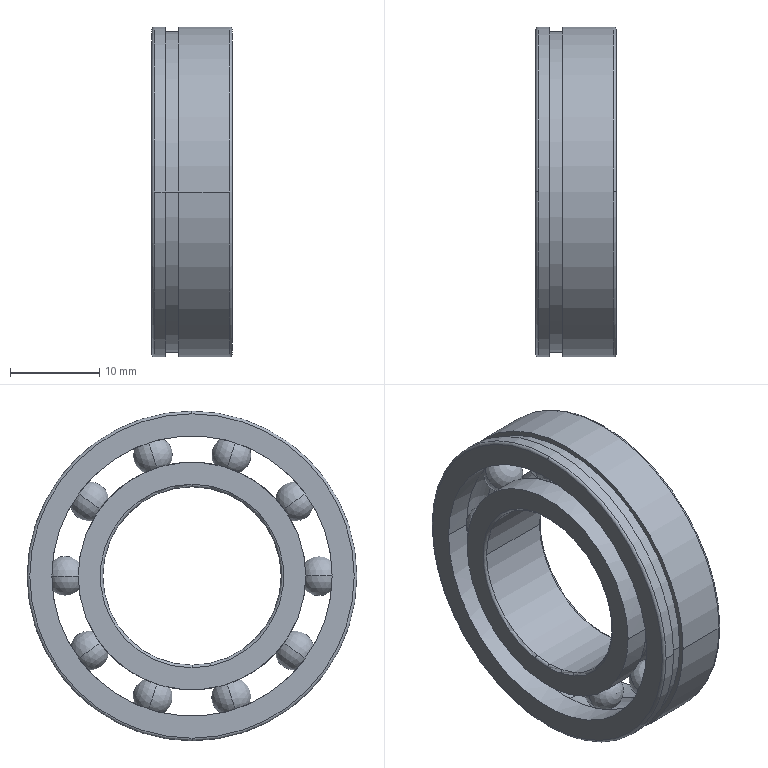Part | SolidWorks | features BaseBody 12 | 12 solids | 56 faces | box 9 x 37 x 37 mm | volume 4521 mm3 | sphere 20 | cylinder 16 | torus 14 | plane 6 | commonest cylinder face diameters 25.542 x4 31.458 x4 37 x4 20 x2 35.92 x2
STEP:
#1=CARTESIAN_POINT('',(4.5,12.04,0.));
#2=VERTEX_POINT('',#1);
#3=CARTESIAN_POINT('',(4.5,16.46,0.));
#4=VERTEX_POINT('',#3);
#5=CARTESIAN_POINT('',(4.5,14.25,0.));
#6=DIRECTION('',(0.,0.,1.));
#7=DIRECTION('',(1.,0.,0.));
#8=AXIS2_PLACEMENT_3D('',#5,#6,#7);
#9=CIRCLE('',#8,2.21);
#10=EDGE_CURVE('',#2,#4,#9,.T.);
#11=ORIENTED_EDGE('',*,*,#10,.F.);
#12=CARTESIAN_POINT('',(4.5,14.25,0.));
#13=DIRECTION('',(0.,0.,-1.));
#14=DIRECTION('',(-1.,0.,0.));
#15=AXIS2_PLACEMENT_3D('',#12,#13,#14);
#16=CIRCLE('',#15,2.21);
#17=EDGE_CURVE('',#2,#4,#16,.T.);
#18=ORIENTED_EDGE('',*,*,#17,.T.);
#19=EDGE_LOOP('',(#11,#18));
#20=FACE_OUTER_BOUND('',#19,.T.);
#21=CARTESIAN_POINT('',(4.5,14.25,0.));
#22=DIRECTION('',(0.,0.,-1.));
#23=DIRECTION('',(1.,0.,0.));
#24=AXIS2_PLACEMENT_3D('',#21,#22,#23);
#25=SPHERICAL_SURFACE('',#24,2.21);
#26=ADVANCED_FACE('',(#20),#25,.T.);
#27=ORIENTED_EDGE('',*,*,#17,.F.);
#28=ORIENTED_EDGE('',*,*,#10,.T.);
#29=EDGE_LOOP('',(#27,#28));
#30=FACE_OUTER_BOUND('',#29,.T.);
#31=CARTESIAN_POINT('',(4.5,14.25,0.));
#32=DIRECTION('',(0.,0.,-1.));
#33=DIRECTION('',(1.,0.,0.));
#34=AXIS2_PLACEMENT_3D('',#31,#32,#33);
#35=SPHERICAL_SURFACE('',#34,2.21);
#36=ADVANCED_FACE('',(#30),#35,.T.);
#37=CLOSED_SHELL('',(#26,#36));
#38=MANIFOLD_SOLID_BREP('',#37);
#39=CARTESIAN_POINT('',(3.,-17.96,0.));
#40=VERTEX_POINT('',#39);
#41=CARTESIAN_POINT('',(3.,17.96,0.));
#42=VERTEX_POINT('',#41);
#43=CARTESIAN_POINT('',(3.,0.,0.));
#44=DIRECTION('',(1.,0.,0.));
#45=DIRECTION('',(0.,1.,0.));
#46=AXIS2_PLACEMENT_3D('',#43,#44,#45);
#47=CIRCLE('',#46,17.96);
#48=EDGE_CURVE('',#40,#42,#47,.T.);
#49=ORIENTED_EDGE('',*,*,#48,.F.);
#50=CARTESIAN_POINT('',(1.5,-17.96,0.));
#51=VERTEX_POINT('',#50);
#52=CARTESIAN_POINT('',(2.25,-17.96,0.));
#53=DIRECTION('',(-1.,0.,0.));
#54=VECTOR('',#53,1000.);
#55=LINE('',#52,#54);
#56=EDGE_CURVE('',#40,#51,#55,.T.);
#57=ORIENTED_EDGE('',*,*,#56,.T.);
#58=CARTESIAN_POINT('',(1.5,17.96,0.));
#59=VERTEX_POINT('',#58);
#60=CARTESIAN_POINT('',(1.5,0.,0.));
#61=DIRECTION('',(1.,0.,0.));
#62=DIRECTION('',(0.,1.,0.));
#63=AXIS2_PLACEMENT_3D('',#60,#61,#62);
#64=CIRCLE('',#63,17.96);
#65=EDGE_CURVE('',#51,#59,#64,.T.);
#66=ORIENTED_EDGE('',*,*,#65,.T.);
#67=CARTESIAN_POINT('',(2.25,17.96,0.));
#68=DIRECTION('',(-1.,0.,0.));
#69=VECTOR('',#68,1000.);
#70=LINE('',#67,#69);
#71=EDGE_CURVE('',#42,#59,#70,.T.);
#72=ORIENTED_EDGE('',*,*,#71,.F.);
#73=EDGE_LOOP('',(#49,#57,#66,#72));
#74=FACE_OUTER_BOUND('',#73,.T.);
#75=CARTESIAN_POINT('',(2.25,0.,0.));
#76=DIRECTION('',(-1.,0.,0.));
#77=DIRECTION('',(0.,1.,0.));
#78=AXIS2_PLACEMENT_3D('',#75,#76,#77);
#79=CYLINDRICAL_SURFACE('',#78,17.96);
#80=ADVANCED_FACE('',(#74),#79,.T.);
#81=CARTESIAN_POINT('',(8.7,-18.5,0.));
#82=VERTEX_POINT('',#81);
#83=CARTESIAN_POINT('',(8.7,0.,-18.5));
#84=VERTEX_POINT('',#83);
#85=CARTESIAN_POINT('',(8.7,0.,0.));
#86=DIRECTION('',(1.,0.,0.));
#87=DIRECTION('',(0.,-1.,0.));
#88=AXIS2_PLACEMENT_3D('',#85,#86,#87);
#89=CIRCLE('',#88,18.5);
#90=EDGE_CURVE('',#82,#84,#89,.T.);
#91=ORIENTED_EDGE('',*,*,#90,.F.);
#92=CARTESIAN_POINT('',(3.,-18.5,0.));
#93=VERTEX_POINT('',#92);
#94=CARTESIAN_POINT('',(6.,-18.5,0.));
#95=DIRECTION('',(-1.,0.,0.));
#96=VECTOR('',#95,1000.);
#97=LINE('',#94,#96);
#98=EDGE_CURVE('',#82,#93,#97,.T.);
#99=ORIENTED_EDGE('',*,*,#98,.T.);
#100=CARTESIAN_POINT('',(3.,18.5,0.));
#101=VERTEX_POINT('',#100);
#102=CARTESIAN_POINT('',(3.,0.,0.));
#103=DIRECTION('',(1.,0.,0.));
#104=DIRECTION('',(0.,1.,0.));
#105=AXIS2_PLACEMENT_3D('',#102,#103,#104);
#106=CIRCLE('',#105,18.5);
#107=EDGE_CURVE('',#93,#101,#106,.T.);
#108=ORIENTED_EDGE('',*,*,#107,.T.);
#109=CARTESIAN_POINT('',(8.7,18.5,0.));
#110=VERTEX_POINT('',#109);
#111=CARTESIAN_POINT('',(6.,18.5,0.));
#112=DIRECTION('',(-1.,0.,0.));
#113=VECTOR('',#112,1000.);
#114=LINE('',#111,#113);
#115=EDGE_CURVE('',#110,#101,#114,.T.);
#116=ORIENTED_EDGE('',*,*,#115,.F.);
#117=CARTESIAN_POINT('',(8.7,0.,0.));
#118=DIRECTION('',(1.,0.,0.));
#119=DIRECTION('',(0.,-1.,0.));
#120=AXIS2_PLACEMENT_3D('',#117,#118,#119);
#121=CIRCLE('',#120,18.5);
#122=EDGE_CURVE('',#84,#110,#121,.T.);
#123=ORIENTED_EDGE('',*,*,#122,.F.);
#124=EDGE_LOOP('',(#91,#99,#108,#116,#123));
#125=FACE_OUTER_BOUND('',#124,.T.);
#126=CARTESIAN_POINT('',(6.,0.,0.));
#127=DIRECTION('',(-1.,0.,0.));
#128=DIRECTION('',(0.,1.,0.));
#129=AXIS2_PLACEMENT_3D('',#126,#127,#128);
#130=CYLINDRICAL_SURFACE('',#129,18.5);
#131=ADVANCED_FACE('',(#125),#130,.T.);
#132=CARTESIAN_POINT('',(1.5,-18.5,0.));
#133=VERTEX_POINT('',#132);
#134=CARTESIAN_POINT('',(1.5,18.5,0.));
#135=VERTEX_POINT('',#134);
#136=CARTESIAN_POINT('',(1.5,0.,0.));
#137=DIRECTION('',(1.,0.,0.));
#138=DIRECTION('',(0.,1.,0.));
#139=AXIS2_PLACEMENT_3D('',#136,#137,#138);
#140=CIRCLE('',#139,18.5);
#141=EDGE_CURVE('',#133,#135,#140,.T.);
#142=ORIENTED_EDGE('',*,*,#141,.F.);
#143=CARTESIAN_POINT('',(0.3,-18.5,0.));
#144=VERTEX_POINT('',#143);
#145=CARTESIAN_POINT('',(0.75,-18.5,0.));
#146=DIRECTION('',(-1.,0.,0.));
#147=VECTOR('',#146,1000.);
#148=LINE('',#145,#147);
#149=EDGE_CURVE('',#133,#144,#148,.T.);
#150=ORIENTED_EDGE('',*,*,#149,.T.);
#151=CARTESIAN_POINT('',(0.3,0.,-18.5));
#152=VERTEX_POINT('',#151);
#153=CARTESIAN_POINT('',(0.3,0.,0.));
#154=DIRECTION('',(-1.,0.,0.));
#155=DIRECTION('',(0.,-1.,0.));
#156=AXIS2_PLACEMENT_3D('',#153,#154,#155);
#157=CIRCLE('',#156,18.5);
#158=EDGE_CURVE('',#152,#144,#157,.T.);
#159=ORIENTED_EDGE('',*,*,#158,.F.);
#160=CARTESIAN_POINT('',(0.3,18.5,0.));
#161=VERTEX_POINT('',#160);
#162=CARTESIAN_POINT('',(0.3,0.,0.));
#163=DIRECTION('',(-1.,0.,0.));
#164=DIRECTION('',(0.,-1.,0.));
#165=AXIS2_PLACEMENT_3D('',#162,#163,#164);
#166=CIRCLE('',#165,18.5);
#167=EDGE_CURVE('',#161,#152,#166,.T.);
#168=ORIENTED_EDGE('',*,*,#167,.F.);
#169=CARTESIAN_POINT('',(0.75,18.5,0.));
#170=DIRECTION('',(-1.,0.,0.));
#171=VECTOR('',#170,1000.);
#172=LINE('',#169,#171);
#173=EDGE_CURVE('',#135,#161,#172,.T.);
#174=ORIENTED_EDGE('',*,*,#173,.F.);
#175=EDGE_LOOP('',(#142,#150,#159,#168,#174));
#176=FACE_OUTER_BOUND('',#175,.T.);
#177=CARTESIAN_POINT('',(0.75,0.,0.));
#178=DIRECTION('',(-1.,0.,0.));
#179=DIRECTION('',(0.,1.,0.));
#180=AXIS2_PLACEMENT_3D('',#177,#178,#179);
#181=CYLINDRICAL_SURFACE('',#180,18.5);
#182=ADVANCED_FACE('',(#176),#181,.T.);
#183=ORIENTED_EDGE('',*,*,#122,.T.);
#184=CARTESIAN_POINT('',(8.7,0.,18.5));
#185=VERTEX_POINT('',#184);
#186=CARTESIAN_POINT('',(8.7,0.,0.));
#187=DIRECTION('',(1.,0.,0.));
#188=DIRECTION('',(0.,-1.,0.));
#189=AXIS2_PLACEMENT_3D('',#186,#187,#188);
#190=CIRCLE('',#189,18.5);
#191=EDGE_CURVE('',#110,#185,#190,.T.);
#192=ORIENTED_EDGE('',*,*,#191,.T.);
#193=CARTESIAN_POINT('',(9.,0.,18.2));
#194=VERTEX_POINT('',#193);
#195=CARTESIAN_POINT('',(8.7,0.,18.2));
#196=DIRECTION('',(0.,1.,0.));
#197=DIRECTION('',(0.,0.,1.));
#198=AXIS2_PLACEMENT_3D('',#195,#196,#197);
#199=CIRCLE('',#198,0.3);
#200=EDGE_CURVE('',#185,#194,#199,.T.);
#201=ORIENTED_EDGE('',*,*,#200,.T.);
#202=CARTESIAN_POINT('',(9.,0.,-18.2));
#203=VERTEX_POINT('',#202);
#204=CARTESIAN_POINT('',(9.,0.,0.));
#205=DIRECTION('',(-1.,0.,0.));
#206=DIRECTION('',(0.,-1.,0.));
#207=AXIS2_PLACEMENT_3D('',#204,#205,#206);
#208=CIRCLE('',#207,18.2);
#209=EDGE_CURVE('',#194,#203,#208,.T.);
#210=ORIENTED_EDGE('',*,*,#209,.T.);
#211=CARTESIAN_POINT('',(8.7,0.,-18.2));
#212=DIRECTION('',(0.,-1.,0.));
#213=DIRECTION('',(0.,0.,-1.));
#214=AXIS2_PLACEMENT_3D('',#211,#212,#213);
#215=CIRCLE('',#214,0.3);
#216=EDGE_CURVE('',#84,#203,#215,.T.);
#217=ORIENTED_EDGE('',*,*,#216,.F.);
#218=EDGE_LOOP('',(#183,#192,#201,#210,#217));
#219=FACE_OUTER_BOUND('',#218,.T.);
#220=CARTESIAN_POINT('',(8.7,0.,0.));
#221=DIRECTION('',(1.,0.,0.));
#222=DIRECTION('',(0.,0.,-1.));
#223=AXIS2_PLACEMENT_3D('',#220,#221,#222);
#224=TOROIDAL_SURFACE('',#223,18.2,0.3);
#225=ADVANCED_FACE('',(#219),#224,.T.);
#226=CARTESIAN_POINT('',(0.,0.,-18.2));
#227=VERTEX_POINT('',#226);
#228=CARTESIAN_POINT('',(0.,0.,18.2));
#229=VERTEX_POINT('',#228);
#230=CARTESIAN_POINT('',(0.,0.,0.));
#231=DIRECTION('',(1.,0.,0.));
#232=DIRECTION('',(0.,-1.,0.));
#233=AXIS2_PLACEMENT_3D('',#230,#231,#232);
#234=CIRCLE('',#233,18.2);
#235=EDGE_CURVE('',#227,#229,#234,.T.);
#236=ORIENTED_EDGE('',*,*,#235,.T.);
#237=CARTESIAN_POINT('',(0.3,0.,18.5));
#238=VERTEX_POINT('',#237);
#239=CARTESIAN_POINT('',(0.3,0.,18.2));
#240=DIRECTION('',(0.,1.,0.));
#241=DIRECTION('',(0.,0.,1.));
#242=AXIS2_PLACEMENT_3D('',#239,#240,#241);
#243=CIRCLE('',#242,0.3);
#244=EDGE_CURVE('',#229,#238,#243,.T.);
#245=ORIENTED_EDGE('',*,*,#244,.T.);
#246=CARTESIAN_POINT('',(0.3,0.,0.));
#247=DIRECTION('',(-1.,0.,0.));
#248=DIRECTION('',(0.,-1.,0.));
#249=AXIS2_PLACEMENT_3D('',#246,#247,#248);
#250=CIRCLE('',#249,18.5);
#251=EDGE_CURVE('',#238,#161,#250,.T.);
#252=ORIENTED_EDGE('',*,*,#251,.T.);
#253=ORIENTED_EDGE('',*,*,#167,.T.);
#254=CARTESIAN_POINT('',(0.3,0.,-18.2));
#255=DIRECTION('',(0.,-1.,0.));
#256=DIRECTION('',(0.,0.,-1.));
#257=AXIS2_PLACEMENT_3D('',#254,#255,#256);
#258=CIRCLE('',#257,0.3);
#259=EDGE_CURVE('',#227,#152,#258,.T.);
#260=ORIENTED_EDGE('',*,*,#259,.F.);
#261=EDGE_LOOP('',(#236,#245,#252,#253,#260));
#262=FACE_OUTER_BOUND('',#261,.T.);
#263=CARTESIAN_POINT('',(0.3,0.,0.));
#264=DIRECTION('',(1.,0.,0.));
#265=DIRECTION('',(0.,0.,-1.));
#266=AXIS2_PLACEMENT_3D('',#263,#264,#265);
#267=TOROIDAL_SURFACE('',#266,18.2,0.3);
#268=ADVANCED_FACE('',(#262),#267,.T.);
#269=CARTESIAN_POINT('',(2.858,0.,15.729));
#270=VERTEX_POINT('',#269);
#271=CARTESIAN_POINT('',(2.858,-15.729,0.));
#272=VERTEX_POINT('',#271);
#273=CARTESIAN_POINT('',(2.858,0.,0.));
#274=DIRECTION('',(1.,0.,0.));
#275=DIRECTION('',(0.,1.,0.));
#276=AXIS2_PLACEMENT_3D('',#273,#274,#275);
#277=CIRCLE('',#276,15.729);
#278=EDGE_CURVE('',#270,#272,#277,.T.);
#279=ORIENTED_EDGE('',*,*,#278,.F.);
#280=CARTESIAN_POINT('',(6.142,0.,15.729));
#281=VERTEX_POINT('',#280);
#282=CARTESIAN_POINT('',(4.5,0.,14.25));
#283=DIRECTION('',(0.,1.,0.));
#284=DIRECTION('',(0.,0.,1.));
#285=AXIS2_PLACEMENT_3D('',#282,#283,#284);
#286=CIRCLE('',#285,2.21);
#287=EDGE_CURVE('',#270,#281,#286,.T.);
#288=ORIENTED_EDGE('',*,*,#287,.T.);
#289=CARTESIAN_POINT('',(6.142,-15.729,0.));
#290=VERTEX_POINT('',#289);
#291=CARTESIAN_POINT('',(6.142,0.,0.));
#292=DIRECTION('',(1.,0.,0.));
#293=DIRECTION('',(0.,1.,0.));
#294=AXIS2_PLACEMENT_3D('',#291,#292,#293);
#295=CIRCLE('',#294,15.729);
#296=EDGE_CURVE('',#281,#290,#295,.T.);
#297=ORIENTED_EDGE('',*,*,#296,.T.);
#298=CARTESIAN_POINT('',(6.142,0.,-15.729));
#299=VERTEX_POINT('',#298);
#300=CARTESIAN_POINT('',(6.142,0.,0.));
#301=DIRECTION('',(1.,0.,0.));
#302=DIRECTION('',(0.,1.,0.));
#303=AXIS2_PLACEMENT_3D('',#300,#301,#302);
#304=CIRCLE('',#303,15.729);
#305=EDGE_CURVE('',#290,#299,#304,.T.);
#306=ORIENTED_EDGE('',*,*,#305,.T.);
#307=CARTESIAN_POINT('',(2.858,0.,-15.729));
#308=VERTEX_POINT('',#307);
#309=CARTESIAN_POINT('',(4.5,0.,-14.25));
#310=DIRECTION('',(0.,-1.,0.));
#311=DIRECTION('',(0.,0.,-1.));
#312=AXIS2_PLACEMENT_3D('',#309,#310,#311);
#313=CIRCLE('',#312,2.21);
#314=EDGE_CURVE('',#308,#299,#313,.T.);
#315=ORIENTED_EDGE('',*,*,#314,.F.);
#316=CARTESIAN_POINT('',(2.858,0.,0.));
#317=DIRECTION('',(1.,0.,0.));
#318=DIRECTION('',(0.,1.,0.));
#319=AXIS2_PLACEMENT_3D('',#316,#317,#318);
#320=CIRCLE('',#319,15.729);
#321=EDGE_CURVE('',#272,#308,#320,.T.);
#322=ORIENTED_EDGE('',*,*,#321,.F.);
#323=EDGE_LOOP('',(#279,#288,#297,#306,#315,#322));
#324=FACE_OUTER_BOUND('',#323,.T.);
#325=CARTESIAN_POINT('',(4.5,0.,0.));
#326=DIRECTION('',(1.,0.,0.));
#327=DIRECTION('',(0.,0.,-1.));
#328=AXIS2_PLACEMENT_3D('',#325,#326,#327);
#329=TOROIDAL_SURFACE('',#328,14.25,2.21);
#330=ADVANCED_FACE('',(#324),#329,.F.);
#331=CARTESIAN_POINT('',(9.,15.729,0.));
#332=VERTEX_POINT('',#331);
#333=CARTESIAN_POINT('',(9.,-15.729,0.));
#334=VERTEX_POINT('',#333);
#335=CARTESIAN_POINT('',(9.,0.,0.));
#336=DIRECTION('',(1.,0.,0.));
#337=DIRECTION('',(0.,1.,0.));
#338=AXIS2_PLACEMENT_3D('',#335,#336,#337);
#339=CIRCLE('',#338,15.729);
#340=EDGE_CURVE('',#332,#334,#339,.T.);
#341=ORIENTED_EDGE('',*,*,#340,.T.);
#342=CARTESIAN_POINT('',(7.571,-15.729,0.));
#343=DIRECTION('',(-1.,0.,0.));
#344=VECTOR('',#343,1000.);
#345=LINE('',#342,#344);
#346=EDGE_CURVE('',#334,#290,#345,.T.);
#347=ORIENTED_EDGE('',*,*,#346,.T.);
#348=ORIENTED_EDGE('',*,*,#296,.F.);
#349=CARTESIAN_POINT('',(6.142,15.729,0.));
#350=VERTEX_POINT('',#349);
#351=CARTESIAN_POINT('',(6.142,0.,0.));
#352=DIRECTION('',(1.,0.,0.));
#353=DIRECTION('',(0.,1.,0.));
#354=AXIS2_PLACEMENT_3D('',#351,#352,#353);
#355=CIRCLE('',#354,15.729);
#356=EDGE_CURVE('',#350,#281,#355,.T.);
#357=ORIENTED_EDGE('',*,*,#356,.F.);
#358=CARTESIAN_POINT('',(7.571,15.729,0.));
#359=DIRECTION('',(-1.,0.,0.));
#360=VECTOR('',#359,1000.);
#361=LINE('',#358,#360);
#362=EDGE_CURVE('',#332,#350,#361,.T.);
#363=ORIENTED_EDGE('',*,*,#362,.F.);
#364=EDGE_LOOP('',(#341,#347,#348,#357,#363));
#365=FACE_OUTER_BOUND('',#364,.T.);
#366=CARTESIAN_POINT('',(7.571,0.,0.));
#367=DIRECTION('',(-1.,0.,0.));
#368=DIRECTION('',(0.,1.,0.));
#369=AXIS2_PLACEMENT_3D('',#366,#367,#368);
#370=CYLINDRICAL_SURFACE('',#369,15.729);
#371=ADVANCED_FACE('',(#365),#370,.F.);
#372=CARTESIAN_POINT('',(2.858,15.729,0.));
#373=VERTEX_POINT('',#372);
#374=CARTESIAN_POINT('',(2.858,0.,0.));
#375=DIRECTION('',(1.,0.,0.));
#376=DIRECTION('',(0.,1.,0.));
#377=AXIS2_PLACEMENT_3D('',#374,#375,#376);
#378=CIRCLE('',#377,15.729);
#379=EDGE_CURVE('',#373,#270,#378,.T.);
#380=ORIENTED_EDGE('',*,*,#379,.T.);
#381=ORIENTED_EDGE('',*,*,#278,.T.);
#382=CARTESIAN_POINT('',(0.,-15.729,0.));
#383=VERTEX_POINT('',#382);
#384=CARTESIAN_POINT('',(1.429,-15.729,0.));
#385=DIRECTION('',(-1.,0.,0.));
#386=VECTOR('',#385,1000.);
#387=LINE('',#384,#386);
#388=EDGE_CURVE('',#272,#383,#387,.T.);
#389=ORIENTED_EDGE('',*,*,#388,.T.);
#390=CARTESIAN_POINT('',(0.,15.729,0.));
#391=VERTEX_POINT('',#390);
#392=CARTESIAN_POINT('',(0.,0.,0.));
#393=DIRECTION('',(1.,0.,0.));
#394=DIRECTION('',(0.,1.,0.));
#395=AXIS2_PLACEMENT_3D('',#392,#393,#394);
#396=CIRCLE('',#395,15.729);
#397=EDGE_CURVE('',#391,#383,#396,.T.);
#398=ORIENTED_EDGE('',*,*,#397,.F.);
#399=CARTESIAN_POINT('',(1.429,15.729,0.));
#400=DIRECTION('',(-1.,0.,0.));
#401=VECTOR('',#400,1000.);
#402=LINE('',#399,#401);
#403=EDGE_CURVE('',#373,#391,#402,.T.);
#404=ORIENTED_EDGE('',*,*,#403,.F.);
#405=EDGE_LOOP('',(#380,#381,#389,#398,#404));
#406=FACE_OUTER_BOUND('',#405,.T.);
#407=CARTESIAN_POINT('',(1.429,0.,0.));
#408=DIRECTION('',(-1.,0.,0.));
#409=DIRECTION('',(0.,1.,0.));
#410=AXIS2_PLACEMENT_3D('',#407,#408,#409);
#411=CYLINDRICAL_SURFACE('',#410,15.729);
#412=ADVANCED_FACE('',(#406),#411,.F.);
#413=CARTESIAN_POINT('',(3.,0.,0.));
#414=DIRECTION('',(1.,0.,0.));
#415=DIRECTION('',(0.,1.,0.));
#416=AXIS2_PLACEMENT_3D('',#413,#414,#415);
#417=CIRCLE('',#416,17.96);
#418=EDGE_CURVE('',#42,#40,#417,.T.);
#419=ORIENTED_EDGE('',*,*,#418,.T.);
#420=ORIENTED_EDGE('',*,*,#48,.T.);
#421=EDGE_LOOP('',(#419,#420));
#422=FACE_BOUND('',#421,.T.);
#423=CARTESIAN_POINT('',(3.,0.,0.));
#424=DIRECTION('',(1.,0.,0.));
#425=DIRECTION('',(0.,1.,0.));
#426=AXIS2_PLACEMENT_3D('',#423,#424,#425);
#427=CIRCLE('',#426,18.5);
#428=EDGE_CURVE('',#101,#93,#427,.T.);
#429=ORIENTED_EDGE('',*,*,#428,.F.);
#430=ORIENTED_EDGE('',*,*,#107,.F.);
#431=EDGE_LOOP('',(#429,#430));
#432=FACE_OUTER_BOUND('',#431,.T.);
#433=CARTESIAN_POINT('',(3.,18.23,0.));
#434=DIRECTION('',(-1.,0.,0.));
#435=DIRECTION('',(0.,0.,1.));
#436=AXIS2_PLACEMENT_3D('',#433,#434,#435);
#437=PLANE('',#436);
#438=ADVANCED_FACE('',(#422,#432),#437,.T.);
#439=CARTESIAN_POINT('',(1.5,0.,0.));
#440=DIRECTION('',(1.,0.,0.));
#441=DIRECTION('',(0.,1.,0.));
#442=AXIS2_PLACEMENT_3D('',#439,#440,#441);
#443=CIRCLE('',#442,17.96);
#444=EDGE_CURVE('',#59,#51,#443,.T.);
#445=ORIENTED_EDGE('',*,*,#444,.F.);
#446=ORIENTED_EDGE('',*,*,#65,.F.);
#447=EDGE_LOOP('',(#445,#446));
#448=FACE_BOUND('',#447,.T.);
#449=CARTESIAN_POINT('',(1.5,0.,0.));
#450=DIRECTION('',(1.,0.,0.));
#451=DIRECTION('',(0.,1.,0.));
#452=AXIS2_PLACEMENT_3D('',#449,#450,#451);
#453=CIRCLE('',#452,18.5);
#454=EDGE_CURVE('',#135,#133,#453,.T.);
#455=ORIENTED_EDGE('',*,*,#454,.T.);
#456=ORIENTED_EDGE('',*,*,#141,.T.);
#457=EDGE_LOOP('',(#455,#456));
#458=FACE_OUTER_BOUND('',#457,.T.);
#459=CARTESIAN_POINT('',(1.5,18.23,0.));
#460=DIRECTION('',(1.,0.,0.));
#461=DIRECTION('',(0.,1.,0.));
#462=AXIS2_PLACEMENT_3D('',#459,#460,#461);
#463=PLANE('',#462);
#464=ADVANCED_FACE('',(#448,#458),#463,.T.);
#465=ORIENTED_EDGE('',*,*,#340,.F.);
#466=CARTESIAN_POINT('',(9.,0.,0.));
#467=DIRECTION('',(1.,0.,0.));
#468=DIRECTION('',(0.,1.,0.));
#469=AXIS2_PLACEMENT_3D('',#466,#467,#468);
#470=CIRCLE('',#469,15.729);
#471=EDGE_CURVE('',#334,#332,#470,.T.);
#472=ORIENTED_EDGE('',*,*,#471,.F.);
#473=EDGE_LOOP('',(#465,#472));
#474=FACE_BOUND('',#473,.T.);
#475=CARTESIAN_POINT('',(9.,0.,0.));
#476=DIRECTION('',(-1.,0.,0.));
#477=DIRECTION('',(0.,-1.,0.));
#478=AXIS2_PLACEMENT_3D('',#475,#476,#477);
#479=CIRCLE('',#478,18.2);
#480=EDGE_CURVE('',#203,#194,#479,.T.);
#481=ORIENTED_EDGE('',*,*,#480,.F.);
#482=ORIENTED_EDGE('',*,*,#209,.F.);
#483=EDGE_LOOP('',(#481,#482));
#484=FACE_OUTER_BOUND('',#483,.T.);
#485=CARTESIAN_POINT('',(9.,17.114,0.));
#486=DIRECTION('',(1.,0.,0.));
#487=DIRECTION('',(0.,1.,0.));
#488=AXIS2_PLACEMENT_3D('',#485,#486,#487);
#489=PLANE('',#488);
#490=ADVANCED_FACE('',(#474,#484),#489,.T.);
#491=ORIENTED_EDGE('',*,*,#397,.T.);
#492=CARTESIAN_POINT('',(0.,0.,0.));
#493=DIRECTION('',(1.,0.,0.));
#494=DIRECTION('',(0.,1.,0.));
#495=AXIS2_PLACEMENT_3D('',#492,#493,#494);
#496=CIRCLE('',#495,15.729);
#497=EDGE_CURVE('',#383,#391,#496,.T.);
#498=ORIENTED_EDGE('',*,*,#497,.T.);
#499=EDGE_LOOP('',(#491,#498));
#500=FACE_BOUND('',#499,.T.);
#501=ORIENTED_EDGE('',*,*,#235,.F.);
#502=CARTESIAN_POINT('',(0.,0.,0.));
#503=DIRECTION('',(1.,0.,0.));
#504=DIRECTION('',(0.,-1.,0.));
#505=AXIS2_PLACEMENT_3D('',#502,#503,#504);
#506=CIRCLE('',#505,18.2);
#507=EDGE_CURVE('',#229,#227,#506,.T.);
#508=ORIENTED_EDGE('',*,*,#507,.F.);
#509=EDGE_LOOP('',(#501,#508));
#510=FACE_OUTER_BOUND('',#509,.T.);
#511=CARTESIAN_POINT('',(0.,17.114,0.));
#512=DIRECTION('',(-1.,0.,0.));
#513=DIRECTION('',(0.,0.,1.));
#514=AXIS2_PLACEMENT_3D('',#511,#512,#513);
#515=PLANE('',#514);
#516=ADVANCED_FACE('',(#500,#510),#515,.T.);
#517=ORIENTED_EDGE('',*,*,#388,.F.);
#518=ORIENTED_EDGE('',*,*,#321,.T.);
#519=CARTESIAN_POINT('',(2.858,0.,0.));
#520=DIRECTION('',(1.,0.,0.));
#521=DIRECTION('',(0.,1.,0.));
#522=AXIS2_PLACEMENT_3D('',#519,#520,#521);
#523=CIRCLE('',#522,15.729);
#524=EDGE_CURVE('',#308,#373,#523,.T.);
#525=ORIENTED_EDGE('',*,*,#524,.T.);
#526=ORIENTED_EDGE('',*,*,#403,.T.);
#527=ORIENTED_EDGE('',*,*,#497,.F.);
#528=EDGE_LOOP('',(#517,#518,#525,#526,#527));
#529=FACE_OUTER_BOUND('',#528,.T.);
#530=CARTESIAN_POINT('',(1.429,0.,0.));
#531=DIRECTION('',(-1.,0.,0.));
#532=DIRECTION('',(0.,1.,0.));
#533=AXIS2_PLACEMENT_3D('',#530,#531,#532);
#534=CYLINDRICAL_SURFACE('',#533,15.729);
#535=ADVANCED_FACE('',(#529),#534,.F.);
#536=ORIENTED_EDGE('',*,*,#346,.F.);
#537=ORIENTED_EDGE('',*,*,#471,.T.);
#538=ORIENTED_EDGE('',*,*,#362,.T.);
#539=CARTESIAN_POINT('',(6.142,0.,0.));
#540=DIRECTION('',(1.,0.,0.));
#541=DIRECTION('',(0.,1.,0.));
#542=AXIS2_PLACEMENT_3D('',#539,#540,#541);
#543=CIRCLE('',#542,15.729);
#544=EDGE_CURVE('',#299,#350,#543,.T.);
#545=ORIENTED_EDGE('',*,*,#544,.F.);
#546=ORIENTED_EDGE('',*,*,#305,.F.);
#547=EDGE_LOOP('',(#536,#537,#538,#545,#546));
#548=FACE_OUTER_BOUND('',#547,.T.);
#549=CARTESIAN_POINT('',(7.571,0.,0.));
#550=DIRECTION('',(-1.,0.,0.));
#551=DIRECTION('',(0.,1.,0.));
#552=AXIS2_PLACEMENT_3D('',#549,#550,#551);
#553=CYLINDRICAL_SURFACE('',#552,15.729);
#554=ADVANCED_FACE('',(#548),#553,.F.);
#555=ORIENTED_EDGE('',*,*,#287,.F.);
#556=ORIENTED_EDGE('',*,*,#379,.F.);
#557=ORIENTED_EDGE('',*,*,#524,.F.);
#558=ORIENTED_EDGE('',*,*,#314,.T.);
#559=ORIENTED_EDGE('',*,*,#544,.T.);
#560=ORIENTED_EDGE('',*,*,#356,.T.);
#561=EDGE_LOOP('',(#555,#556,#557,#558,#559,#560));
#562=FACE_OUTER_BOUND('',#561,.T.);
#563=CARTESIAN_POINT('',(4.5,0.,0.));
#564=DIRECTION('',(1.,0.,0.));
#565=DIRECTION('',(0.,0.,-1.));
#566=AXIS2_PLACEMENT_3D('',#563,#564,#565);
#567=TOROIDAL_SURFACE('',#566,14.25,2.21);
#568=ADVANCED_FACE('',(#562),#567,.F.);
#569=ORIENTED_EDGE('',*,*,#244,.F.);
#570=ORIENTED_EDGE('',*,*,#507,.T.);
#571=ORIENTED_EDGE('',*,*,#259,.T.);
#572=ORIENTED_EDGE('',*,*,#158,.T.);
#573=CARTESIAN_POINT('',(0.3,0.,0.));
#574=DIRECTION('',(-1.,0.,0.));
#575=DIRECTION('',(0.,-1.,0.));
#576=AXIS2_PLACEMENT_3D('',#573,#574,#575);
#577=CIRCLE('',#576,18.5);
#578=EDGE_CURVE('',#144,#238,#577,.T.);
#579=ORIENTED_EDGE('',*,*,#578,.T.);
#580=EDGE_LOOP('',(#569,#570,#571,#572,#579));
#581=FACE_OUTER_BOUND('',#580,.T.);
#582=CARTESIAN_POINT('',(0.3,0.,0.));
#583=DIRECTION('',(1.,0.,0.));
#584=DIRECTION('',(0.,0.,-1.));
#585=AXIS2_PLACEMENT_3D('',#582,#583,#584);
#586=TOROIDAL_SURFACE('',#585,18.2,0.3);
#587=ADVANCED_FACE('',(#581),#586,.T.);
#588=ORIENTED_EDGE('',*,*,#200,.F.);
#589=CARTESIAN_POINT('',(8.7,0.,0.));
#590=DIRECTION('',(1.,0.,0.));
#591=DIRECTION('',(0.,-1.,0.));
#592=AXIS2_PLACEMENT_3D('',#589,#590,#591);
#593=CIRCLE('',#592,18.5);
#594=EDGE_CURVE('',#185,#82,#593,.T.);
#595=ORIENTED_EDGE('',*,*,#594,.T.);
#596=ORIENTED_EDGE('',*,*,#90,.T.);
#597=ORIENTED_EDGE('',*,*,#216,.T.);
#598=ORIENTED_EDGE('',*,*,#480,.T.);
#599=EDGE_LOOP('',(#588,#595,#596,#597,#598));
#600=FACE_OUTER_BOUND('',#599,.T.);
#601=CARTESIAN_POINT('',(8.7,0.,0.));
#602=DIRECTION('',(1.,0.,0.));
#603=DIRECTION('',(0.,0.,-1.));
#604=AXIS2_PLACEMENT_3D('',#601,#602,#603);
#605=TOROIDAL_SURFACE('',#604,18.2,0.3);
#606=ADVANCED_FACE('',(#600),#605,.T.);
#607=ORIENTED_EDGE('',*,*,#149,.F.);
#608=ORIENTED_EDGE('',*,*,#454,.F.);
#609=ORIENTED_EDGE('',*,*,#173,.T.);
#610=ORIENTED_EDGE('',*,*,#251,.F.);
#611=ORIENTED_EDGE('',*,*,#578,.F.);
#612=EDGE_LOOP('',(#607,#608,#609,#610,#611));
#613=FACE_OUTER_BOUND('',#612,.T.);
#614=CARTESIAN_POINT('',(0.75,0.,0.));
#615=DIRECTION('',(-1.,0.,0.));
#616=DIRECTION('',(0.,1.,0.));
#617=AXIS2_PLACEMENT_3D('',#614,#615,#616);
#618=CYLINDRICAL_SURFACE('',#617,18.5);
#619=ADVANCED_FACE('',(#613),#618,.T.);
#620=ORIENTED_EDGE('',*,*,#98,.F.);
#621=ORIENTED_EDGE('',*,*,#594,.F.);
#622=ORIENTED_EDGE('',*,*,#191,.F.);
#623=ORIENTED_EDGE('',*,*,#115,.T.);
#624=ORIENTED_EDGE('',*,*,#428,.T.);
#625=EDGE_LOOP('',(#620,#621,#622,#623,#624));
#626=FACE_OUTER_BOUND('',#625,.T.);
#627=CARTESIAN_POINT('',(6.,0.,0.));
#628=DIRECTION('',(-1.,0.,0.));
#629=DIRECTION('',(0.,1.,0.));
#630=AXIS2_PLACEMENT_3D('',#627,#628,#629);
#631=CYLINDRICAL_SURFACE('',#630,18.5);
#632=ADVANCED_FACE('',(#626),#631,.T.);
#633=ORIENTED_EDGE('',*,*,#56,.F.);
#634=ORIENTED_EDGE('',*,*,#418,.F.);
#635=ORIENTED_EDGE('',*,*,#71,.T.);
#636=ORIENTED_EDGE('',*,*,#444,.T.);
#637=EDGE_LOOP('',(#633,#634,#635,#636));
#638=FACE_OUTER_BOUND('',#637,.T.);
#639=CARTESIAN_POINT('',(2.25,0.,0.));
#640=DIRECTION('',(-1.,0.,0.));
#641=DIRECTION('',(0.,1.,0.));
#642=AXIS2_PLACEMENT_3D('',#639,#640,#641);
#643=CYLINDRICAL_SURFACE('',#642,17.96);
#644=ADVANCED_FACE('',(#638),#643,.T.);
#645=CLOSED_SHELL('',(#80,#131,#182,#225,#268,#330,#371,#412,#438,#464,#490,#516,#535,#554,#568,#587,#606,#619,#632,#644));
#646=MANIFOLD_SOLID_BREP('',#645);
#647=CARTESIAN_POINT('',(6.142,0.,-12.771));
#648=VERTEX_POINT('',#647);
#649=CARTESIAN_POINT('',(4.5,0.,-12.04));
#650=VERTEX_POINT('',#649);
#651=CARTESIAN_POINT('',(4.5,0.,-14.25));
#652=DIRECTION('',(0.,-1.,0.));
#653=DIRECTION('',(0.,0.,-1.));
#654=AXIS2_PLACEMENT_3D('',#651,#652,#653);
#655=CIRCLE('',#654,2.21);
#656=EDGE_CURVE('',#648,#650,#655,.T.);
#657=ORIENTED_EDGE('',*,*,#656,.T.);
#658=CARTESIAN_POINT('',(4.5,0.,12.04));
#659=VERTEX_POINT('',#658);
#660=CARTESIAN_POINT('',(4.5,0.,0.));
#661=DIRECTION('',(1.,0.,0.));
#662=DIRECTION('',(0.,0.,-1.));
#663=AXIS2_PLACEMENT_3D('',#660,#661,#662);
#664=CIRCLE('',#663,12.04);
#665=EDGE_CURVE('',#650,#659,#664,.T.);
#666=ORIENTED_EDGE('',*,*,#665,.T.);
#667=CARTESIAN_POINT('',(6.142,0.,12.771));
#668=VERTEX_POINT('',#667);
#669=CARTESIAN_POINT('',(4.5,0.,14.25));
#670=DIRECTION('',(0.,1.,0.));
#671=DIRECTION('',(0.,0.,1.));
#672=AXIS2_PLACEMENT_3D('',#669,#670,#671);
#673=CIRCLE('',#672,2.21);
#674=EDGE_CURVE('',#668,#659,#673,.T.);
#675=ORIENTED_EDGE('',*,*,#674,.F.);
#676=CARTESIAN_POINT('',(6.142,12.771,0.));
#677=VERTEX_POINT('',#676);
#678=CARTESIAN_POINT('',(6.142,0.,0.));
#679=DIRECTION('',(1.,0.,0.));
#680=DIRECTION('',(0.,1.,0.));
#681=AXIS2_PLACEMENT_3D('',#678,#679,#680);
#682=CIRCLE('',#681,12.771);
#683=EDGE_CURVE('',#677,#668,#682,.T.);
#684=ORIENTED_EDGE('',*,*,#683,.F.);
#685=CARTESIAN_POINT('',(6.142,0.,0.));
#686=DIRECTION('',(1.,0.,0.));
#687=DIRECTION('',(0.,1.,0.));
#688=AXIS2_PLACEMENT_3D('',#685,#686,#687);
#689=CIRCLE('',#688,12.771);
#690=EDGE_CURVE('',#648,#677,#689,.T.);
#691=ORIENTED_EDGE('',*,*,#690,.F.);
#692=EDGE_LOOP('',(#657,#666,#675,#684,#691));
#693=FACE_OUTER_BOUND('',#692,.T.);
#694=CARTESIAN_POINT('',(4.5,0.,0.));
#695=DIRECTION('',(1.,0.,0.));
#696=DIRECTION('',(0.,0.,-1.));
#697=AXIS2_PLACEMENT_3D('',#694,#695,#696);
#698=TOROIDAL_SURFACE('',#697,14.25,2.21);
#699=ADVANCED_FACE('',(#693),#698,.F.);
#700=ORIENTED_EDGE('',*,*,#674,.T.);
#701=CARTESIAN_POINT('',(4.5,0.,0.));
#702=DIRECTION('',(1.,0.,0.));
#703=DIRECTION('',(0.,0.,-1.));
#704=AXIS2_PLACEMENT_3D('',#701,#702,#703);
#705=CIRCLE('',#704,12.04);
#706=EDGE_CURVE('',#659,#650,#705,.T.);
#707=ORIENTED_EDGE('',*,*,#706,.T.);
#708=ORIENTED_EDGE('',*,*,#656,.F.);
#709=CARTESIAN_POINT('',(6.142,-12.771,0.));
#710=VERTEX_POINT('',#709);
#711=CARTESIAN_POINT('',(6.142,0.,0.));
#712=DIRECTION('',(1.,0.,0.));
#713=DIRECTION('',(0.,1.,0.));
#714=AXIS2_PLACEMENT_3D('',#711,#712,#713);
#715=CIRCLE('',#714,12.771);
#716=EDGE_CURVE('',#710,#648,#715,.T.);
#717=ORIENTED_EDGE('',*,*,#716,.F.);
#718=CARTESIAN_POINT('',(6.142,0.,0.));
#719=DIRECTION('',(1.,0.,0.));
#720=DIRECTION('',(0.,1.,0.));
#721=AXIS2_PLACEMENT_3D('',#718,#719,#720);
#722=CIRCLE('',#721,12.771);
#723=EDGE_CURVE('',#668,#710,#722,.T.);
#724=ORIENTED_EDGE('',*,*,#723,.F.);
#725=EDGE_LOOP('',(#700,#707,#708,#717,#724));
#726=FACE_OUTER_BOUND('',#725,.T.);
#727=CARTESIAN_POINT('',(4.5,0.,0.));
#728=DIRECTION('',(1.,0.,0.));
#729=DIRECTION('',(0.,0.,-1.));
#730=AXIS2_PLACEMENT_3D('',#727,#728,#729);
#731=TOROIDAL_SURFACE('',#730,14.25,2.21);
#732=ADVANCED_FACE('',(#726),#731,.F.);
#733=ORIENTED_EDGE('',*,*,#706,.F.);
#734=CARTESIAN_POINT('',(2.858,0.,12.771));
#735=VERTEX_POINT('',#734);
#736=CARTESIAN_POINT('',(4.5,0.,14.25));
#737=DIRECTION('',(0.,1.,0.));
#738=DIRECTION('',(0.,0.,1.));
#739=AXIS2_PLACEMENT_3D('',#736,#737,#738);
#740=CIRCLE('',#739,2.21);
#741=EDGE_CURVE('',#659,#735,#740,.T.);
#742=ORIENTED_EDGE('',*,*,#741,.T.);
#743=CARTESIAN_POINT('',(2.858,-12.771,0.));
#744=VERTEX_POINT('',#743);
#745=CARTESIAN_POINT('',(2.858,0.,0.));
#746=DIRECTION('',(1.,0.,0.));
#747=DIRECTION('',(0.,1.,0.));
#748=AXIS2_PLACEMENT_3D('',#745,#746,#747);
#749=CIRCLE('',#748,12.771);
#750=EDGE_CURVE('',#735,#744,#749,.T.);
#751=ORIENTED_EDGE('',*,*,#750,.T.);
#752=CARTESIAN_POINT('',(2.858,0.,-12.771));
#753=VERTEX_POINT('',#752);
#754=CARTESIAN_POINT('',(2.858,0.,0.));
#755=DIRECTION('',(1.,0.,0.));
#756=DIRECTION('',(0.,1.,0.));
#757=AXIS2_PLACEMENT_3D('',#754,#755,#756);
#758=CIRCLE('',#757,12.771);
#759=EDGE_CURVE('',#744,#753,#758,.T.);
#760=ORIENTED_EDGE('',*,*,#759,.T.);
#761=CARTESIAN_POINT('',(4.5,0.,-14.25));
#762=DIRECTION('',(0.,-1.,0.));
#763=DIRECTION('',(0.,0.,-1.));
#764=AXIS2_PLACEMENT_3D('',#761,#762,#763);
#765=CIRCLE('',#764,2.21);
#766=EDGE_CURVE('',#650,#753,#765,.T.);
#767=ORIENTED_EDGE('',*,*,#766,.F.);
#768=EDGE_LOOP('',(#733,#742,#751,#760,#767));
#769=FACE_OUTER_BOUND('',#768,.T.);
#770=CARTESIAN_POINT('',(4.5,0.,0.));
#771=DIRECTION('',(1.,0.,0.));
#772=DIRECTION('',(0.,0.,-1.));
#773=AXIS2_PLACEMENT_3D('',#770,#771,#772);
#774=TOROIDAL_SURFACE('',#773,14.25,2.21);
#775=ADVANCED_FACE('',(#769),#774,.F.);
#776=CARTESIAN_POINT('',(8.7,-10.,0.));
#777=VERTEX_POINT('',#776);
#778=CARTESIAN_POINT('',(8.7,0.,10.));
#779=VERTEX_POINT('',#778);
#780=CARTESIAN_POINT('',(8.7,0.,0.));
#781=DIRECTION('',(-1.,0.,0.));
#782=DIRECTION('',(0.,-1.,0.));
#783=AXIS2_PLACEMENT_3D('',#780,#781,#782);
#784=CIRCLE('',#783,10.);
#785=EDGE_CURVE('',#777,#779,#784,.T.);
#786=ORIENTED_EDGE('',*,*,#785,.F.);
#787=CARTESIAN_POINT('',(0.3,-10.,0.));
#788=VERTEX_POINT('',#787);
#789=CARTESIAN_POINT('',(4.5,-10.,0.));
#790=DIRECTION('',(-1.,0.,0.));
#791=VECTOR('',#790,1000.);
#792=LINE('',#789,#791);
#793=EDGE_CURVE('',#777,#788,#792,.T.);
#794=ORIENTED_EDGE('',*,*,#793,.T.);
#795=CARTESIAN_POINT('',(0.3,0.,10.));
#796=VERTEX_POINT('',#795);
#797=CARTESIAN_POINT('',(0.3,0.,0.));
#798=DIRECTION('',(1.,0.,0.));
#799=DIRECTION('',(0.,-1.,0.));
#800=AXIS2_PLACEMENT_3D('',#797,#798,#799);
#801=CIRCLE('',#800,10.);
#802=EDGE_CURVE('',#796,#788,#801,.T.);
#803=ORIENTED_EDGE('',*,*,#802,.F.);
#804=CARTESIAN_POINT('',(0.3,10.,0.));
#805=VERTEX_POINT('',#804);
#806=CARTESIAN_POINT('',(0.3,0.,0.));
#807=DIRECTION('',(1.,0.,0.));
#808=DIRECTION('',(0.,-1.,0.));
#809=AXIS2_PLACEMENT_3D('',#806,#807,#808);
#810=CIRCLE('',#809,10.);
#811=EDGE_CURVE('',#805,#796,#810,.T.);
#812=ORIENTED_EDGE('',*,*,#811,.F.);
#813=CARTESIAN_POINT('',(8.7,10.,0.));
#814=VERTEX_POINT('',#813);
#815=CARTESIAN_POINT('',(4.5,10.,0.));
#816=DIRECTION('',(-1.,0.,0.));
#817=VECTOR('',#816,1000.);
#818=LINE('',#815,#817);
#819=EDGE_CURVE('',#814,#805,#818,.T.);
#820=ORIENTED_EDGE('',*,*,#819,.F.);
#821=CARTESIAN_POINT('',(8.7,0.,0.));
#822=DIRECTION('',(-1.,0.,0.));
#823=DIRECTION('',(0.,-1.,0.));
#824=AXIS2_PLACEMENT_3D('',#821,#822,#823);
#825=CIRCLE('',#824,10.);
#826=EDGE_CURVE('',#779,#814,#825,.T.);
#827=ORIENTED_EDGE('',*,*,#826,.F.);
#828=EDGE_LOOP('',(#786,#794,#803,#812,#820,#827));
#829=FACE_OUTER_BOUND('',#828,.T.);
#830=CARTESIAN_POINT('',(4.5,0.,0.));
#831=DIRECTION('',(-1.,0.,0.));
#832=DIRECTION('',(0.,1.,0.));
#833=AXIS2_PLACEMENT_3D('',#830,#831,#832);
#834=CYLINDRICAL_SURFACE('',#833,10.);
#835=ADVANCED_FACE('',(#829),#834,.F.);
#836=CARTESIAN_POINT('',(0.3,0.,-10.));
#837=VERTEX_POINT('',#836);
#838=CARTESIAN_POINT('',(0.3,0.,0.));
#839=DIRECTION('',(1.,0.,0.));
#840=DIRECTION('',(0.,-1.,0.));
#841=AXIS2_PLACEMENT_3D('',#838,#839,#840);
#842=CIRCLE('',#841,10.);
#843=EDGE_CURVE('',#837,#805,#842,.T.);
#844=ORIENTED_EDGE('',*,*,#843,.T.);
#845=ORIENTED_EDGE('',*,*,#811,.T.);
#846=CARTESIAN_POINT('',(0.,0.,10.3));
#847=VERTEX_POINT('',#846);
#848=CARTESIAN_POINT('',(0.3,0.,10.3));
#849=DIRECTION('',(0.,1.,0.));
#850=DIRECTION('',(0.,0.,1.));
#851=AXIS2_PLACEMENT_3D('',#848,#849,#850);
#852=CIRCLE('',#851,0.3);
#853=EDGE_CURVE('',#796,#847,#852,.T.);
#854=ORIENTED_EDGE('',*,*,#853,.T.);
#855=CARTESIAN_POINT('',(0.,0.,-10.3));
#856=VERTEX_POINT('',#855);
#857=CARTESIAN_POINT('',(0.,0.,0.));
#858=DIRECTION('',(-1.,0.,0.));
#859=DIRECTION('',(0.,-1.,0.));
#860=AXIS2_PLACEMENT_3D('',#857,#858,#859);
#861=CIRCLE('',#860,10.3);
#862=EDGE_CURVE('',#847,#856,#861,.T.);
#863=ORIENTED_EDGE('',*,*,#862,.T.);
#864=CARTESIAN_POINT('',(0.3,0.,-10.3));
#865=DIRECTION('',(0.,-1.,0.));
#866=DIRECTION('',(0.,0.,-1.));
#867=AXIS2_PLACEMENT_3D('',#864,#865,#866);
#868=CIRCLE('',#867,0.3);
#869=EDGE_CURVE('',#837,#856,#868,.T.);
#870=ORIENTED_EDGE('',*,*,#869,.F.);
#871=EDGE_LOOP('',(#844,#845,#854,#863,#870));
#872=FACE_OUTER_BOUND('',#871,.T.);
#873=CARTESIAN_POINT('',(0.3,0.,0.));
#874=DIRECTION('',(1.,0.,0.));
#875=DIRECTION('',(0.,0.,-1.));
#876=AXIS2_PLACEMENT_3D('',#873,#874,#875);
#877=TOROIDAL_SURFACE('',#876,10.3,0.3);
#878=ADVANCED_FACE('',(#872),#877,.T.);
#879=CARTESIAN_POINT('',(9.,0.,-10.3));
#880=VERTEX_POINT('',#879);
#881=CARTESIAN_POINT('',(9.,0.,10.3));
#882=VERTEX_POINT('',#881);
#883=CARTESIAN_POINT('',(9.,0.,0.));
#884=DIRECTION('',(1.,0.,0.));
#885=DIRECTION('',(0.,-1.,0.));
#886=AXIS2_PLACEMENT_3D('',#883,#884,#885);
#887=CIRCLE('',#886,10.3);
#888=EDGE_CURVE('',#880,#882,#887,.T.);
#889=ORIENTED_EDGE('',*,*,#888,.T.);
#890=CARTESIAN_POINT('',(8.7,0.,10.3));
#891=DIRECTION('',(0.,1.,0.));
#892=DIRECTION('',(0.,0.,1.));
#893=AXIS2_PLACEMENT_3D('',#890,#891,#892);
#894=CIRCLE('',#893,0.3);
#895=EDGE_CURVE('',#882,#779,#894,.T.);
#896=ORIENTED_EDGE('',*,*,#895,.T.);
#897=ORIENTED_EDGE('',*,*,#826,.T.);
#898=CARTESIAN_POINT('',(8.7,0.,-10.));
#899=VERTEX_POINT('',#898);
#900=CARTESIAN_POINT('',(8.7,0.,0.));
#901=DIRECTION('',(-1.,0.,0.));
#902=DIRECTION('',(0.,-1.,0.));
#903=AXIS2_PLACEMENT_3D('',#900,#901,#902);
#904=CIRCLE('',#903,10.);
#905=EDGE_CURVE('',#814,#899,#904,.T.);
#906=ORIENTED_EDGE('',*,*,#905,.T.);
#907=CARTESIAN_POINT('',(8.7,0.,-10.3));
#908=DIRECTION('',(0.,-1.,0.));
#909=DIRECTION('',(0.,0.,-1.));
#910=AXIS2_PLACEMENT_3D('',#907,#908,#909);
#911=CIRCLE('',#910,0.3);
#912=EDGE_CURVE('',#880,#899,#911,.T.);
#913=ORIENTED_EDGE('',*,*,#912,.F.);
#914=EDGE_LOOP('',(#889,#896,#897,#906,#913));
#915=FACE_OUTER_BOUND('',#914,.T.);
#916=CARTESIAN_POINT('',(8.7,0.,0.));
#917=DIRECTION('',(1.,0.,0.));
#918=DIRECTION('',(0.,0.,-1.));
#919=AXIS2_PLACEMENT_3D('',#916,#917,#918);
#920=TOROIDAL_SURFACE('',#919,10.3,0.3);
#921=ADVANCED_FACE('',(#915),#920,.T.);
#922=ORIENTED_EDGE('',*,*,#759,.F.);
#923=CARTESIAN_POINT('',(0.,-12.771,0.));
#924=VERTEX_POINT('',#923);
#925=CARTESIAN_POINT('',(1.429,-12.771,0.));
#926=DIRECTION('',(-1.,0.,0.));
#927=VECTOR('',#926,1000.);
#928=LINE('',#925,#927);
#929=EDGE_CURVE('',#744,#924,#928,.T.);
#930=ORIENTED_EDGE('',*,*,#929,.T.);
#931=CARTESIAN_POINT('',(0.,12.771,0.));
#932=VERTEX_POINT('',#931);
#933=CARTESIAN_POINT('',(0.,0.,0.));
#934=DIRECTION('',(1.,0.,0.));
#935=DIRECTION('',(0.,1.,0.));
#936=AXIS2_PLACEMENT_3D('',#933,#934,#935);
#937=CIRCLE('',#936,12.771);
#938=EDGE_CURVE('',#924,#932,#937,.T.);
#939=ORIENTED_EDGE('',*,*,#938,.T.);
#940=CARTESIAN_POINT('',(2.858,12.771,0.));
#941=VERTEX_POINT('',#940);
#942=CARTESIAN_POINT('',(1.429,12.771,0.));
#943=DIRECTION('',(-1.,0.,0.));
#944=VECTOR('',#943,1000.);
#945=LINE('',#942,#944);
#946=EDGE_CURVE('',#941,#932,#945,.T.);
#947=ORIENTED_EDGE('',*,*,#946,.F.);
#948=CARTESIAN_POINT('',(2.858,0.,0.));
#949=DIRECTION('',(1.,0.,0.));
#950=DIRECTION('',(0.,1.,0.));
#951=AXIS2_PLACEMENT_3D('',#948,#949,#950);
#952=CIRCLE('',#951,12.771);
#953=EDGE_CURVE('',#753,#941,#952,.T.);
#954=ORIENTED_EDGE('',*,*,#953,.F.);
#955=EDGE_LOOP('',(#922,#930,#939,#947,#954));
#956=FACE_OUTER_BOUND('',#955,.T.);
#957=CARTESIAN_POINT('',(1.429,0.,0.));
#958=DIRECTION('',(-1.,0.,0.));
#959=DIRECTION('',(0.,1.,0.));
#960=AXIS2_PLACEMENT_3D('',#957,#958,#959);
#961=CYLINDRICAL_SURFACE('',#960,12.771);
#962=ADVANCED_FACE('',(#956),#961,.T.);
#963=CARTESIAN_POINT('',(9.,-12.771,0.));
#964=VERTEX_POINT('',#963);
#965=CARTESIAN_POINT('',(9.,12.771,0.));
#966=VERTEX_POINT('',#965);
#967=CARTESIAN_POINT('',(9.,0.,0.));
#968=DIRECTION('',(1.,0.,0.));
#969=DIRECTION('',(0.,1.,0.));
#970=AXIS2_PLACEMENT_3D('',#967,#968,#969);
#971=CIRCLE('',#970,12.771);
#972=EDGE_CURVE('',#964,#966,#971,.T.);
#973=ORIENTED_EDGE('',*,*,#972,.F.);
#974=CARTESIAN_POINT('',(7.571,-12.771,0.));
#975=DIRECTION('',(-1.,0.,0.));
#976=VECTOR('',#975,1000.);
#977=LINE('',#974,#976);
#978=EDGE_CURVE('',#964,#710,#977,.T.);
#979=ORIENTED_EDGE('',*,*,#978,.T.);
#980=ORIENTED_EDGE('',*,*,#716,.T.);
#981=ORIENTED_EDGE('',*,*,#690,.T.);
#982=CARTESIAN_POINT('',(7.571,12.771,0.));
#983=DIRECTION('',(-1.,0.,0.));
#984=VECTOR('',#983,1000.);
#985=LINE('',#982,#984);
#986=EDGE_CURVE('',#966,#677,#985,.T.);
#987=ORIENTED_EDGE('',*,*,#986,.F.);
#988=EDGE_LOOP('',(#973,#979,#980,#981,#987));
#989=FACE_OUTER_BOUND('',#988,.T.);
#990=CARTESIAN_POINT('',(7.571,0.,0.));
#991=DIRECTION('',(-1.,0.,0.));
#992=DIRECTION('',(0.,1.,0.));
#993=AXIS2_PLACEMENT_3D('',#990,#991,#992);
#994=CYLINDRICAL_SURFACE('',#993,12.771);
#995=ADVANCED_FACE('',(#989),#994,.T.);
#996=CARTESIAN_POINT('',(0.,0.,0.));
#997=DIRECTION('',(-1.,0.,0.));
#998=DIRECTION('',(0.,-1.,0.));
#999=AXIS2_PLACEMENT_3D('',#996,#997,#998);
#1000=CIRCLE('',#999,10.3);
#1001=EDGE_CURVE('',#856,#847,#1000,.T.);
#1002=ORIENTED_EDGE('',*,*,#1001,.F.);
#1003=ORIENTED_EDGE('',*,*,#862,.F.);
#1004=EDGE_LOOP('',(#1002,#1003));
#1005=FACE_BOUND('',#1004,.T.);
#1006=CARTESIAN_POINT('',(0.,0.,0.));
#1007=DIRECTION('',(1.,0.,0.));
#1008=DIRECTION('',(0.,1.,0.));
#1009=AXIS2_PLACEMENT_3D('',#1006,#1007,#1008);
#1010=CIRCLE('',#1009,12.771);
#1011=EDGE_CURVE('',#932,#924,#1010,.T.);
#1012=ORIENTED_EDGE('',*,*,#1011,.F.);
#1013=ORIENTED_EDGE('',*,*,#938,.F.);
#1014=EDGE_LOOP('',(#1012,#1013));
#1015=FACE_OUTER_BOUND('',#1014,.T.);
#1016=CARTESIAN_POINT('',(0.,11.386,0.));
#1017=DIRECTION('',(-1.,0.,0.));
#1018=DIRECTION('',(0.,0.,1.));
#1019=AXIS2_PLACEMENT_3D('',#1016,#1017,#1018);
#1020=PLANE('',#1019);
#1021=ADVANCED_FACE('',(#1005,#1015),#1020,.T.);
#1022=ORIENTED_EDGE('',*,*,#888,.F.);
#1023=CARTESIAN_POINT('',(9.,0.,0.));
#1024=DIRECTION('',(1.,0.,0.));
#1025=DIRECTION('',(0.,-1.,0.));
#1026=AXIS2_PLACEMENT_3D('',#1023,#1024,#1025);
#1027=CIRCLE('',#1026,10.3);
#1028=EDGE_CURVE('',#882,#880,#1027,.T.);
#1029=ORIENTED_EDGE('',*,*,#1028,.F.);
#1030=EDGE_LOOP('',(#1022,#1029));
#1031=FACE_BOUND('',#1030,.T.);
#1032=CARTESIAN_POINT('',(9.,0.,0.));
#1033=DIRECTION('',(1.,0.,0.));
#1034=DIRECTION('',(0.,1.,0.));
#1035=AXIS2_PLACEMENT_3D('',#1032,#1033,#1034);
#1036=CIRCLE('',#1035,12.771);
#1037=EDGE_CURVE('',#966,#964,#1036,.T.);
#1038=ORIENTED_EDGE('',*,*,#1037,.T.);
#1039=ORIENTED_EDGE('',*,*,#972,.T.);
#1040=EDGE_LOOP('',(#1038,#1039));
#1041=FACE_OUTER_BOUND('',#1040,.T.);
#1042=CARTESIAN_POINT('',(9.,11.386,0.));
#1043=DIRECTION('',(1.,0.,0.));
#1044=DIRECTION('',(0.,1.,0.));
#1045=AXIS2_PLACEMENT_3D('',#1042,#1043,#1044);
#1046=PLANE('',#1045);
#1047=ADVANCED_FACE('',(#1031,#1041),#1046,.T.);
#1048=ORIENTED_EDGE('',*,*,#978,.F.);
#1049=ORIENTED_EDGE('',*,*,#1037,.F.);
#1050=ORIENTED_EDGE('',*,*,#986,.T.);
#1051=ORIENTED_EDGE('',*,*,#683,.T.);
#1052=ORIENTED_EDGE('',*,*,#723,.T.);
#1053=EDGE_LOOP('',(#1048,#1049,#1050,#1051,#1052));
#1054=FACE_OUTER_BOUND('',#1053,.T.);
#1055=CARTESIAN_POINT('',(7.571,0.,0.));
#1056=DIRECTION('',(-1.,0.,0.));
#1057=DIRECTION('',(0.,1.,0.));
#1058=AXIS2_PLACEMENT_3D('',#1055,#1056,#1057);
#1059=CYLINDRICAL_SURFACE('',#1058,12.771);
#1060=ADVANCED_FACE('',(#1054),#1059,.T.);
#1061=ORIENTED_EDGE('',*,*,#929,.F.);
#1062=ORIENTED_EDGE('',*,*,#750,.F.);
#1063=CARTESIAN_POINT('',(2.858,0.,0.));
#1064=DIRECTION('',(1.,0.,0.));
#1065=DIRECTION('',(0.,1.,0.));
#1066=AXIS2_PLACEMENT_3D('',#1063,#1064,#1065);
#1067=CIRCLE('',#1066,12.771);
#1068=EDGE_CURVE('',#941,#735,#1067,.T.);
#1069=ORIENTED_EDGE('',*,*,#1068,.F.);
#1070=ORIENTED_EDGE('',*,*,#946,.T.);
#1071=ORIENTED_EDGE('',*,*,#1011,.T.);
#1072=EDGE_LOOP('',(#1061,#1062,#1069,#1070,#1071));
#1073=FACE_OUTER_BOUND('',#1072,.T.);
#1074=CARTESIAN_POINT('',(1.429,0.,0.));
#1075=DIRECTION('',(-1.,0.,0.));
#1076=DIRECTION('',(0.,1.,0.));
#1077=AXIS2_PLACEMENT_3D('',#1074,#1075,#1076);
#1078=CYLINDRICAL_SURFACE('',#1077,12.771);
#1079=ADVANCED_FACE('',(#1073),#1078,.T.);
#1080=ORIENTED_EDGE('',*,*,#895,.F.);
#1081=ORIENTED_EDGE('',*,*,#1028,.T.);
#1082=ORIENTED_EDGE('',*,*,#912,.T.);
#1083=CARTESIAN_POINT('',(8.7,0.,0.));
#1084=DIRECTION('',(-1.,0.,0.));
#1085=DIRECTION('',(0.,-1.,0.));
#1086=AXIS2_PLACEMENT_3D('',#1083,#1084,#1085);
#1087=CIRCLE('',#1086,10.);
#1088=EDGE_CURVE('',#899,#777,#1087,.T.);
#1089=ORIENTED_EDGE('',*,*,#1088,.T.);
#1090=ORIENTED_EDGE('',*,*,#785,.T.);
#1091=EDGE_LOOP('',(#1080,#1081,#1082,#1089,#1090));
#1092=FACE_OUTER_BOUND('',#1091,.T.);
#1093=CARTESIAN_POINT('',(8.7,0.,0.));
#1094=DIRECTION('',(1.,0.,0.));
#1095=DIRECTION('',(0.,0.,-1.));
#1096=AXIS2_PLACEMENT_3D('',#1093,#1094,#1095);
#1097=TOROIDAL_SURFACE('',#1096,10.3,0.3);
#1098=ADVANCED_FACE('',(#1092),#1097,.T.);
#1099=ORIENTED_EDGE('',*,*,#853,.F.);
#1100=ORIENTED_EDGE('',*,*,#802,.T.);
#1101=CARTESIAN_POINT('',(0.3,0.,0.));
#1102=DIRECTION('',(1.,0.,0.));
#1103=DIRECTION('',(0.,-1.,0.));
#1104=AXIS2_PLACEMENT_3D('',#1101,#1102,#1103);
#1105=CIRCLE('',#1104,10.);
#1106=EDGE_CURVE('',#788,#837,#1105,.T.);
#1107=ORIENTED_EDGE('',*,*,#1106,.T.);
#1108=ORIENTED_EDGE('',*,*,#869,.T.);
#1109=ORIENTED_EDGE('',*,*,#1001,.T.);
#1110=EDGE_LOOP('',(#1099,#1100,#1107,#1108,#1109));
#1111=FACE_OUTER_BOUND('',#1110,.T.);
#1112=CARTESIAN_POINT('',(0.3,0.,0.));
#1113=DIRECTION('',(1.,0.,0.));
#1114=DIRECTION('',(0.,0.,-1.));
#1115=AXIS2_PLACEMENT_3D('',#1112,#1113,#1114);
#1116=TOROIDAL_SURFACE('',#1115,10.3,0.3);
#1117=ADVANCED_FACE('',(#1111),#1116,.T.);
#1118=ORIENTED_EDGE('',*,*,#793,.F.);
#1119=ORIENTED_EDGE('',*,*,#1088,.F.);
#1120=ORIENTED_EDGE('',*,*,#905,.F.);
#1121=ORIENTED_EDGE('',*,*,#819,.T.);
#1122=ORIENTED_EDGE('',*,*,#843,.F.);
#1123=ORIENTED_EDGE('',*,*,#1106,.F.);
#1124=EDGE_LOOP('',(#1118,#1119,#1120,#1121,#1122,#1123));
#1125=FACE_OUTER_BOUND('',#1124,.T.);
#1126=CARTESIAN_POINT('',(4.5,0.,0.));
#1127=DIRECTION('',(-1.,0.,0.));
#1128=DIRECTION('',(0.,1.,0.));
#1129=AXIS2_PLACEMENT_3D('',#1126,#1127,#1128);
#1130=CYLINDRICAL_SURFACE('',#1129,10.);
#1131=ADVANCED_FACE('',(#1125),#1130,.F.);
#1132=ORIENTED_EDGE('',*,*,#665,.F.);
#1133=ORIENTED_EDGE('',*,*,#766,.T.);
#1134=ORIENTED_EDGE('',*,*,#953,.T.);
#1135=ORIENTED_EDGE('',*,*,#1068,.T.);
#1136=ORIENTED_EDGE('',*,*,#741,.F.);
#1137=EDGE_LOOP('',(#1132,#1133,#1134,#1135,#1136));
#1138=FACE_OUTER_BOUND('',#1137,.T.);
#1139=CARTESIAN_POINT('',(4.5,0.,0.));
#1140=DIRECTION('',(1.,0.,0.));
#1141=DIRECTION('',(0.,0.,-1.));
#1142=AXIS2_PLACEMENT_3D('',#1139,#1140,#1141);
#1143=TOROIDAL_SURFACE('',#1142,14.25,2.21);
#1144=ADVANCED_FACE('',(#1138),#1143,.F.);
#1145=CLOSED_SHELL('',(#699,#732,#775,#835,#878,#921,#962,#995,#1021,#1047,#1060,#1079,#1098,#1117,#1131,#1144));
#1146=MANIFOLD_SOLID_BREP('',#1145);
#1147=CARTESIAN_POINT('',(4.5,9.741,7.077));
#1148=VERTEX_POINT('',#1147);
#1149=CARTESIAN_POINT('',(4.5,13.316,9.675));
#1150=VERTEX_POINT('',#1149);
#1151=CARTESIAN_POINT('',(4.5,11.528,8.376));
#1152=DIRECTION('',(0.,-0.5878,0.809));
#1153=DIRECTION('',(0.,-0.809,-0.5878));
#1154=AXIS2_PLACEMENT_3D('',#1151,#1152,#1153);
#1155=CIRCLE('',#1154,2.21);
#1156=EDGE_CURVE('',#1148,#1150,#1155,.T.);
#1157=ORIENTED_EDGE('',*,*,#1156,.F.);
#1158=CARTESIAN_POINT('',(4.5,11.528,8.376));
#1159=DIRECTION('',(0.,0.5878,-0.809));
#1160=DIRECTION('',(0.,0.809,0.5878));
#1161=AXIS2_PLACEMENT_3D('',#1158,#1159,#1160);
#1162=CIRCLE('',#1161,2.21);
#1163=EDGE_CURVE('',#1148,#1150,#1162,.T.);
#1164=ORIENTED_EDGE('',*,*,#1163,.T.);
#1165=EDGE_LOOP('',(#1157,#1164));
#1166=FACE_OUTER_BOUND('',#1165,.T.);
#1167=CARTESIAN_POINT('',(4.5,11.528,8.376));
#1168=DIRECTION('',(0.,0.5878,-0.809));
#1169=DIRECTION('',(1.,0.,0.));
#1170=AXIS2_PLACEMENT_3D('',#1167,#1168,#1169);
#1171=SPHERICAL_SURFACE('',#1170,2.21);
#1172=ADVANCED_FACE('',(#1166),#1171,.T.);
#1173=ORIENTED_EDGE('',*,*,#1163,.F.);
#1174=ORIENTED_EDGE('',*,*,#1156,.T.);
#1175=EDGE_LOOP('',(#1173,#1174));
#1176=FACE_OUTER_BOUND('',#1175,.T.);
#1177=CARTESIAN_POINT('',(4.5,11.528,8.376));
#1178=DIRECTION('',(0.,0.5878,-0.809));
#1179=DIRECTION('',(1.,0.,0.));
#1180=AXIS2_PLACEMENT_3D('',#1177,#1178,#1179);
#1181=SPHERICAL_SURFACE('',#1180,2.21);
#1182=ADVANCED_FACE('',(#1176),#1181,.T.);
#1183=CLOSED_SHELL('',(#1172,#1182));
#1184=MANIFOLD_SOLID_BREP('',#1183);
#1185=CARTESIAN_POINT('',(4.5,3.721,11.451));
#1186=VERTEX_POINT('',#1185);
#1187=CARTESIAN_POINT('',(4.5,5.086,15.654));
#1188=VERTEX_POINT('',#1187);
#1189=CARTESIAN_POINT('',(4.5,4.403,13.553));
#1190=DIRECTION('',(0.,-0.9511,0.309));
#1191=DIRECTION('',(0.,-0.309,-0.9511));
#1192=AXIS2_PLACEMENT_3D('',#1189,#1190,#1191);
#1193=CIRCLE('',#1192,2.21);
#1194=EDGE_CURVE('',#1186,#1188,#1193,.T.);
#1195=ORIENTED_EDGE('',*,*,#1194,.F.);
#1196=CARTESIAN_POINT('',(4.5,4.403,13.553));
#1197=DIRECTION('',(0.,0.9511,-0.309));
#1198=DIRECTION('',(0.,0.309,0.9511));
#1199=AXIS2_PLACEMENT_3D('',#1196,#1197,#1198);
#1200=CIRCLE('',#1199,2.21);
#1201=EDGE_CURVE('',#1186,#1188,#1200,.T.);
#1202=ORIENTED_EDGE('',*,*,#1201,.T.);
#1203=EDGE_LOOP('',(#1195,#1202));
#1204=FACE_OUTER_BOUND('',#1203,.T.);
#1205=CARTESIAN_POINT('',(4.5,4.403,13.553));
#1206=DIRECTION('',(0.,0.9511,-0.309));
#1207=DIRECTION('',(1.,0.,0.));
#1208=AXIS2_PLACEMENT_3D('',#1205,#1206,#1207);
#1209=SPHERICAL_SURFACE('',#1208,2.21);
#1210=ADVANCED_FACE('',(#1204),#1209,.T.);
#1211=ORIENTED_EDGE('',*,*,#1201,.F.);
#1212=ORIENTED_EDGE('',*,*,#1194,.T.);
#1213=EDGE_LOOP('',(#1211,#1212));
#1214=FACE_OUTER_BOUND('',#1213,.T.);
#1215=CARTESIAN_POINT('',(4.5,4.403,13.553));
#1216=DIRECTION('',(0.,0.9511,-0.309));
#1217=DIRECTION('',(1.,0.,0.));
#1218=AXIS2_PLACEMENT_3D('',#1215,#1216,#1217);
#1219=SPHERICAL_SURFACE('',#1218,2.21);
#1220=ADVANCED_FACE('',(#1214),#1219,.T.);
#1221=CLOSED_SHELL('',(#1210,#1220));
#1222=MANIFOLD_SOLID_BREP('',#1221);
#1223=CARTESIAN_POINT('',(4.5,-3.721,11.451));
#1224=VERTEX_POINT('',#1223);
#1225=CARTESIAN_POINT('',(4.5,-5.086,15.654));
#1226=VERTEX_POINT('',#1225);
#1227=CARTESIAN_POINT('',(4.5,-4.403,13.553));
#1228=DIRECTION('',(0.,-0.9511,-0.309));
#1229=DIRECTION('',(0.,0.309,-0.9511));
#1230=AXIS2_PLACEMENT_3D('',#1227,#1228,#1229);
#1231=CIRCLE('',#1230,2.21);
#1232=EDGE_CURVE('',#1224,#1226,#1231,.T.);
#1233=ORIENTED_EDGE('',*,*,#1232,.F.);
#1234=CARTESIAN_POINT('',(4.5,-4.403,13.553));
#1235=DIRECTION('',(0.,0.9511,0.309));
#1236=DIRECTION('',(0.,-0.309,0.9511));
#1237=AXIS2_PLACEMENT_3D('',#1234,#1235,#1236);
#1238=CIRCLE('',#1237,2.21);
#1239=EDGE_CURVE('',#1224,#1226,#1238,.T.);
#1240=ORIENTED_EDGE('',*,*,#1239,.T.);
#1241=EDGE_LOOP('',(#1233,#1240));
#1242=FACE_OUTER_BOUND('',#1241,.T.);
#1243=CARTESIAN_POINT('',(4.5,-4.403,13.553));
#1244=DIRECTION('',(0.,0.9511,0.309));
#1245=DIRECTION('',(1.,0.,0.));
#1246=AXIS2_PLACEMENT_3D('',#1243,#1244,#1245);
#1247=SPHERICAL_SURFACE('',#1246,2.21);
#1248=ADVANCED_FACE('',(#1242),#1247,.T.);
#1249=ORIENTED_EDGE('',*,*,#1239,.F.);
#1250=ORIENTED_EDGE('',*,*,#1232,.T.);
#1251=EDGE_LOOP('',(#1249,#1250));
#1252=FACE_OUTER_BOUND('',#1251,.T.);
#1253=CARTESIAN_POINT('',(4.5,-4.403,13.553));
#1254=DIRECTION('',(0.,0.9511,0.309));
#1255=DIRECTION('',(1.,0.,0.));
#1256=AXIS2_PLACEMENT_3D('',#1253,#1254,#1255);
#1257=SPHERICAL_SURFACE('',#1256,2.21);
#1258=ADVANCED_FACE('',(#1252),#1257,.T.);
#1259=CLOSED_SHELL('',(#1248,#1258));
#1260=MANIFOLD_SOLID_BREP('',#1259);
#1261=CARTESIAN_POINT('',(4.5,-9.741,7.077));
#1262=VERTEX_POINT('',#1261);
#1263=CARTESIAN_POINT('',(4.5,-13.316,9.675));
#1264=VERTEX_POINT('',#1263);
#1265=CARTESIAN_POINT('',(4.5,-11.528,8.376));
#1266=DIRECTION('',(0.,-0.5878,-0.809));
#1267=DIRECTION('',(0.,0.809,-0.5878));
#1268=AXIS2_PLACEMENT_3D('',#1265,#1266,#1267);
#1269=CIRCLE('',#1268,2.21);
#1270=EDGE_CURVE('',#1262,#1264,#1269,.T.);
#1271=ORIENTED_EDGE('',*,*,#1270,.F.);
#1272=CARTESIAN_POINT('',(4.5,-11.528,8.376));
#1273=DIRECTION('',(0.,0.5878,0.809));
#1274=DIRECTION('',(0.,-0.809,0.5878));
#1275=AXIS2_PLACEMENT_3D('',#1272,#1273,#1274);
#1276=CIRCLE('',#1275,2.21);
#1277=EDGE_CURVE('',#1262,#1264,#1276,.T.);
#1278=ORIENTED_EDGE('',*,*,#1277,.T.);
#1279=EDGE_LOOP('',(#1271,#1278));
#1280=FACE_OUTER_BOUND('',#1279,.T.);
#1281=CARTESIAN_POINT('',(4.5,-11.528,8.376));
#1282=DIRECTION('',(0.,0.5878,0.809));
#1283=DIRECTION('',(1.,0.,0.));
#1284=AXIS2_PLACEMENT_3D('',#1281,#1282,#1283);
#1285=SPHERICAL_SURFACE('',#1284,2.21);
#1286=ADVANCED_FACE('',(#1280),#1285,.T.);
#1287=ORIENTED_EDGE('',*,*,#1277,.F.);
#1288=ORIENTED_EDGE('',*,*,#1270,.T.);
#1289=EDGE_LOOP('',(#1287,#1288));
#1290=FACE_OUTER_BOUND('',#1289,.T.);
#1291=CARTESIAN_POINT('',(4.5,-11.528,8.376));
#1292=DIRECTION('',(0.,0.5878,0.809));
#1293=DIRECTION('',(1.,0.,0.));
#1294=AXIS2_PLACEMENT_3D('',#1291,#1292,#1293);
#1295=SPHERICAL_SURFACE('',#1294,2.21);
#1296=ADVANCED_FACE('',(#1290),#1295,.T.);
#1297=CLOSED_SHELL('',(#1286,#1296));
#1298=MANIFOLD_SOLID_BREP('',#1297);
#1299=CARTESIAN_POINT('',(4.5,-12.04,0.));
#1300=VERTEX_POINT('',#1299);
#1301=CARTESIAN_POINT('',(4.5,-16.46,0.));
#1302=VERTEX_POINT('',#1301);
#1303=CARTESIAN_POINT('',(4.5,-14.25,0.));
#1304=DIRECTION('',(0.,0.,-1.));
#1305=DIRECTION('',(0.,1.,0.));
#1306=AXIS2_PLACEMENT_3D('',#1303,#1304,#1305);
#1307=CIRCLE('',#1306,2.21);
#1308=EDGE_CURVE('',#1300,#1302,#1307,.T.);
#1309=ORIENTED_EDGE('',*,*,#1308,.F.);
#1310=CARTESIAN_POINT('',(4.5,-14.25,0.));
#1311=DIRECTION('',(0.,0.,1.));
#1312=DIRECTION('',(1.,0.,0.));
#1313=AXIS2_PLACEMENT_3D('',#1310,#1311,#1312);
#1314=CIRCLE('',#1313,2.21);
#1315=EDGE_CURVE('',#1300,#1302,#1314,.T.);
#1316=ORIENTED_EDGE('',*,*,#1315,.T.);
#1317=EDGE_LOOP('',(#1309,#1316));
#1318=FACE_OUTER_BOUND('',#1317,.T.);
#1319=CARTESIAN_POINT('',(4.5,-14.25,0.));
#1320=DIRECTION('',(0.,0.,1.));
#1321=DIRECTION('',(1.,0.,0.));
#1322=AXIS2_PLACEMENT_3D('',#1319,#1320,#1321);
#1323=SPHERICAL_SURFACE('',#1322,2.21);
#1324=ADVANCED_FACE('',(#1318),#1323,.T.);
#1325=ORIENTED_EDGE('',*,*,#1315,.F.);
#1326=ORIENTED_EDGE('',*,*,#1308,.T.);
#1327=EDGE_LOOP('',(#1325,#1326));
#1328=FACE_OUTER_BOUND('',#1327,.T.);
#1329=CARTESIAN_POINT('',(4.5,-14.25,0.));
#1330=DIRECTION('',(0.,0.,1.));
#1331=DIRECTION('',(1.,0.,0.));
#1332=AXIS2_PLACEMENT_3D('',#1329,#1330,#1331);
#1333=SPHERICAL_SURFACE('',#1332,2.21);
#1334=ADVANCED_FACE('',(#1328),#1333,.T.);
#1335=CLOSED_SHELL('',(#1324,#1334));
#1336=MANIFOLD_SOLID_BREP('',#1335);
#1337=CARTESIAN_POINT('',(4.5,-9.741,-7.077));
#1338=VERTEX_POINT('',#1337);
#1339=CARTESIAN_POINT('',(4.5,-13.316,-9.675));
#1340=VERTEX_POINT('',#1339);
#1341=CARTESIAN_POINT('',(4.5,-11.528,-8.376));
#1342=DIRECTION('',(0.,0.5878,-0.809));
#1343=DIRECTION('',(0.,0.809,0.5878));
#1344=AXIS2_PLACEMENT_3D('',#1341,#1342,#1343);
#1345=CIRCLE('',#1344,2.21);
#1346=EDGE_CURVE('',#1338,#1340,#1345,.T.);
#1347=ORIENTED_EDGE('',*,*,#1346,.F.);
#1348=CARTESIAN_POINT('',(4.5,-11.528,-8.376));
#1349=DIRECTION('',(0.,-0.5878,0.809));
#1350=DIRECTION('',(0.,-0.809,-0.5878));
#1351=AXIS2_PLACEMENT_3D('',#1348,#1349,#1350);
#1352=CIRCLE('',#1351,2.21);
#1353=EDGE_CURVE('',#1338,#1340,#1352,.T.);
#1354=ORIENTED_EDGE('',*,*,#1353,.T.);
#1355=EDGE_LOOP('',(#1347,#1354));
#1356=FACE_OUTER_BOUND('',#1355,.T.);
#1357=CARTESIAN_POINT('',(4.5,-11.528,-8.376));
#1358=DIRECTION('',(0.,-0.5878,0.809));
#1359=DIRECTION('',(1.,0.,0.));
#1360=AXIS2_PLACEMENT_3D('',#1357,#1358,#1359);
#1361=SPHERICAL_SURFACE('',#1360,2.21);
#1362=ADVANCED_FACE('',(#1356),#1361,.T.);
#1363=ORIENTED_EDGE('',*,*,#1353,.F.);
#1364=ORIENTED_EDGE('',*,*,#1346,.T.);
#1365=EDGE_LOOP('',(#1363,#1364));
#1366=FACE_OUTER_BOUND('',#1365,.T.);
#1367=CARTESIAN_POINT('',(4.5,-11.528,-8.376));
#1368=DIRECTION('',(0.,-0.5878,0.809));
#1369=DIRECTION('',(1.,0.,0.));
#1370=AXIS2_PLACEMENT_3D('',#1367,#1368,#1369);
#1371=SPHERICAL_SURFACE('',#1370,2.21);
#1372=ADVANCED_FACE('',(#1366),#1371,.T.);
#1373=CLOSED_SHELL('',(#1362,#1372));
#1374=MANIFOLD_SOLID_BREP('',#1373);
#1375=CARTESIAN_POINT('',(4.5,-3.721,-11.451));
#1376=VERTEX_POINT('',#1375);
#1377=CARTESIAN_POINT('',(4.5,-5.086,-15.654));
#1378=VERTEX_POINT('',#1377);
#1379=CARTESIAN_POINT('',(4.5,-4.403,-13.553));
#1380=DIRECTION('',(0.,0.9511,-0.309));
#1381=DIRECTION('',(0.,0.309,0.9511));
#1382=AXIS2_PLACEMENT_3D('',#1379,#1380,#1381);
#1383=CIRCLE('',#1382,2.21);
#1384=EDGE_CURVE('',#1376,#1378,#1383,.T.);
#1385=ORIENTED_EDGE('',*,*,#1384,.F.);
#1386=CARTESIAN_POINT('',(4.5,-4.403,-13.553));
#1387=DIRECTION('',(0.,-0.9511,0.309));
#1388=DIRECTION('',(0.,-0.309,-0.9511));
#1389=AXIS2_PLACEMENT_3D('',#1386,#1387,#1388);
#1390=CIRCLE('',#1389,2.21);
#1391=EDGE_CURVE('',#1376,#1378,#1390,.T.);
#1392=ORIENTED_EDGE('',*,*,#1391,.T.);
#1393=EDGE_LOOP('',(#1385,#1392));
#1394=FACE_OUTER_BOUND('',#1393,.T.);
#1395=CARTESIAN_POINT('',(4.5,-4.403,-13.553));
#1396=DIRECTION('',(0.,-0.9511,0.309));
#1397=DIRECTION('',(1.,0.,0.));
#1398=AXIS2_PLACEMENT_3D('',#1395,#1396,#1397);
#1399=SPHERICAL_SURFACE('',#1398,2.21);
#1400=ADVANCED_FACE('',(#1394),#1399,.T.);
#1401=ORIENTED_EDGE('',*,*,#1391,.F.);
#1402=ORIENTED_EDGE('',*,*,#1384,.T.);
#1403=EDGE_LOOP('',(#1401,#1402));
#1404=FACE_OUTER_BOUND('',#1403,.T.);
#1405=CARTESIAN_POINT('',(4.5,-4.403,-13.553));
#1406=DIRECTION('',(0.,-0.9511,0.309));
#1407=DIRECTION('',(1.,0.,0.));
#1408=AXIS2_PLACEMENT_3D('',#1405,#1406,#1407);
#1409=SPHERICAL_SURFACE('',#1408,2.21);
#1410=ADVANCED_FACE('',(#1404),#1409,.T.);
#1411=CLOSED_SHELL('',(#1400,#1410));
#1412=MANIFOLD_SOLID_BREP('',#1411);
#1413=CARTESIAN_POINT('',(4.5,3.721,-11.451));
#1414=VERTEX_POINT('',#1413);
#1415=CARTESIAN_POINT('',(4.5,5.086,-15.654));
#1416=VERTEX_POINT('',#1415);
#1417=CARTESIAN_POINT('',(4.5,4.403,-13.553));
#1418=DIRECTION('',(0.,0.9511,0.309));
#1419=DIRECTION('',(0.,-0.309,0.9511));
#1420=AXIS2_PLACEMENT_3D('',#1417,#1418,#1419);
#1421=CIRCLE('',#1420,2.21);
#1422=EDGE_CURVE('',#1414,#1416,#1421,.T.);
#1423=ORIENTED_EDGE('',*,*,#1422,.F.);
#1424=CARTESIAN_POINT('',(4.5,4.403,-13.553));
#1425=DIRECTION('',(0.,-0.9511,-0.309));
#1426=DIRECTION('',(0.,0.309,-0.9511));
#1427=AXIS2_PLACEMENT_3D('',#1424,#1425,#1426);
#1428=CIRCLE('',#1427,2.21);
#1429=EDGE_CURVE('',#1414,#1416,#1428,.T.);
#1430=ORIENTED_EDGE('',*,*,#1429,.T.);
#1431=EDGE_LOOP('',(#1423,#1430));
#1432=FACE_OUTER_BOUND('',#1431,.T.);
#1433=CARTESIAN_POINT('',(4.5,4.403,-13.553));
#1434=DIRECTION('',(0.,-0.9511,-0.309));
#1435=DIRECTION('',(1.,0.,0.));
#1436=AXIS2_PLACEMENT_3D('',#1433,#1434,#1435);
#1437=SPHERICAL_SURFACE('',#1436,2.21);
#1438=ADVANCED_FACE('',(#1432),#1437,.T.);
#1439=ORIENTED_EDGE('',*,*,#1429,.F.);
#1440=ORIENTED_EDGE('',*,*,#1422,.T.);
#1441=EDGE_LOOP('',(#1439,#1440));
#1442=FACE_OUTER_BOUND('',#1441,.T.);
#1443=CARTESIAN_POINT('',(4.5,4.403,-13.553));
#1444=DIRECTION('',(0.,-0.9511,-0.309));
#1445=DIRECTION('',(1.,0.,0.));
#1446=AXIS2_PLACEMENT_3D('',#1443,#1444,#1445);
#1447=SPHERICAL_SURFACE('',#1446,2.21);
#1448=ADVANCED_FACE('',(#1442),#1447,.T.);
#1449=CLOSED_SHELL('',(#1438,#1448));
#1450=MANIFOLD_SOLID_BREP('',#1449);
#1451=CARTESIAN_POINT('',(4.5,9.741,-7.077));
#1452=VERTEX_POINT('',#1451);
#1453=CARTESIAN_POINT('',(4.5,13.316,-9.675));
#1454=VERTEX_POINT('',#1453);
#1455=CARTESIAN_POINT('',(4.5,11.528,-8.376));
#1456=DIRECTION('',(0.,0.5878,0.809));
#1457=DIRECTION('',(0.,-0.809,0.5878));
#1458=AXIS2_PLACEMENT_3D('',#1455,#1456,#1457);
#1459=CIRCLE('',#1458,2.21);
#1460=EDGE_CURVE('',#1452,#1454,#1459,.T.);
#1461=ORIENTED_EDGE('',*,*,#1460,.F.);
#1462=CARTESIAN_POINT('',(4.5,11.528,-8.376));
#1463=DIRECTION('',(0.,-0.5878,-0.809));
#1464=DIRECTION('',(0.,0.809,-0.5878));
#1465=AXIS2_PLACEMENT_3D('',#1462,#1463,#1464);
#1466=CIRCLE('',#1465,2.21);
#1467=EDGE_CURVE('',#1452,#1454,#1466,.T.);
#1468=ORIENTED_EDGE('',*,*,#1467,.T.);
#1469=EDGE_LOOP('',(#1461,#1468));
#1470=FACE_OUTER_BOUND('',#1469,.T.);
#1471=CARTESIAN_POINT('',(4.5,11.528,-8.376));
#1472=DIRECTION('',(0.,-0.5878,-0.809));
#1473=DIRECTION('',(1.,0.,0.));
#1474=AXIS2_PLACEMENT_3D('',#1471,#1472,#1473);
#1475=SPHERICAL_SURFACE('',#1474,2.21);
#1476=ADVANCED_FACE('',(#1470),#1475,.T.);
#1477=ORIENTED_EDGE('',*,*,#1467,.F.);
#1478=ORIENTED_EDGE('',*,*,#1460,.T.);
#1479=EDGE_LOOP('',(#1477,#1478));
#1480=FACE_OUTER_BOUND('',#1479,.T.);
#1481=CARTESIAN_POINT('',(4.5,11.528,-8.376));
#1482=DIRECTION('',(0.,-0.5878,-0.809));
#1483=DIRECTION('',(1.,0.,0.));
#1484=AXIS2_PLACEMENT_3D('',#1481,#1482,#1483);
#1485=SPHERICAL_SURFACE('',#1484,2.21);
#1486=ADVANCED_FACE('',(#1480),#1485,.T.);
#1487=CLOSED_SHELL('',(#1476,#1486));
#1488=MANIFOLD_SOLID_BREP('',#1487);
#1489=CARTESIAN_POINT('',(0.,0.,0.));
#1490=DIRECTION('',(0.,0.,1.));
#1491=DIRECTION('',(1.,0.,0.));
#1492=AXIS2_PLACEMENT_3D('',#1489,#1490,#1491);
#1493=(LENGTH_UNIT()NAMED_UNIT(*)SI_UNIT(.MILLI.,.METRE.));
#1494=UNCERTAINTY_MEASURE_WITH_UNIT(LENGTH_MEASURE(0.00001),#1493,'','');
#1495=(NAMED_UNIT(*)PLANE_ANGLE_UNIT()SI_UNIT($,.RADIAN.));
#1496=(NAMED_UNIT(*)SI_UNIT($,.STERADIAN.)SOLID_ANGLE_UNIT());
#1497=(GEOMETRIC_REPRESENTATION_CONTEXT(3)GLOBAL_UNCERTAINTY_ASSIGNED_CONTEXT((#1494))GLOBAL_UNIT_ASSIGNED_CONTEXT((#1493,#1495,#1496))REPRESENTATION_CONTEXT('',''));
#1498=ADVANCED_BREP_SHAPE_REPRESENTATION('',(#38,#646,#1146,#1184,#1222,#1260,#1298,#1336,#1374,#1412,#1450,#1488,#1492),#1497);